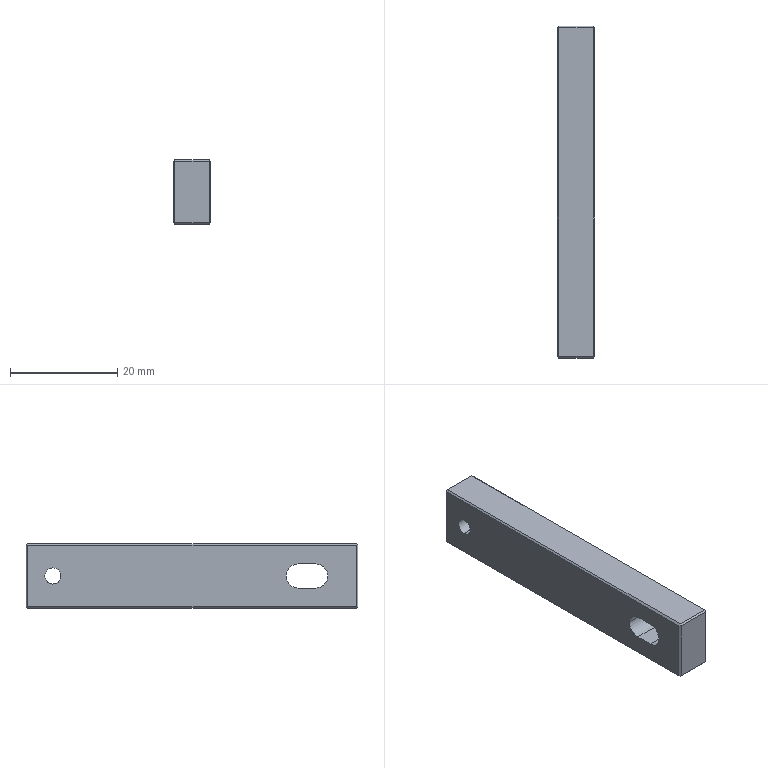Part | NX | 1 solid | 31 faces | box 7 x 62 x 12 mm | volume 4905 mm3 | plane 20 | cylinder 7 | cone 4 | commonest cylinder face diameters 4.5 x3 2.5 x2 3 x2
STEP:
#1=CARTESIAN_POINT('',(-76.,244.,-48.063));
#2=VERTEX_POINT('',#1);
#3=CARTESIAN_POINT('',(-76.,305.4,-48.063));
#4=VERTEX_POINT('',#3);
#5=CARTESIAN_POINT('',(-76.,274.7,-48.063));
#6=DIRECTION('',(0.,1.,0.));
#7=VECTOR('',#6,1000.);
#8=LINE('',#5,#7);
#9=EDGE_CURVE('',#2,#4,#8,.T.);
#10=ORIENTED_EDGE('',*,*,#9,.T.);
#11=CARTESIAN_POINT('',(-76.,305.4,-36.663));
#12=VERTEX_POINT('',#11);
#13=CARTESIAN_POINT('',(-76.,305.4,-42.363));
#14=DIRECTION('',(0.,0.,-1.));
#15=VECTOR('',#14,1000.);
#16=LINE('',#13,#15);
#17=EDGE_CURVE('',#12,#4,#16,.T.);
#18=ORIENTED_EDGE('',*,*,#17,.F.);
#19=CARTESIAN_POINT('',(-76.,244.,-36.663));
#20=VERTEX_POINT('',#19);
#21=CARTESIAN_POINT('',(-76.,274.7,-36.663));
#22=DIRECTION('',(0.,1.,0.));
#23=VECTOR('',#22,1000.);
#24=LINE('',#21,#23);
#25=EDGE_CURVE('',#20,#12,#24,.T.);
#26=ORIENTED_EDGE('',*,*,#25,.F.);
#27=CARTESIAN_POINT('',(-76.,244.,-42.363));
#28=DIRECTION('',(0.,0.,-1.));
#29=VECTOR('',#28,1000.);
#30=LINE('',#27,#29);
#31=EDGE_CURVE('',#20,#2,#30,.T.);
#32=ORIENTED_EDGE('',*,*,#31,.T.);
#33=EDGE_LOOP('',(#10,#18,#26,#32));
#34=FACE_BOUND('',#33,.T.);
#35=CARTESIAN_POINT('',(-76.,251.55,-44.613));
#36=VERTEX_POINT('',#35);
#37=CARTESIAN_POINT('',(-76.,254.85,-44.613));
#38=VERTEX_POINT('',#37);
#39=CARTESIAN_POINT('',(-76.,245.7,-44.613));
#40=DIRECTION('',(0.,1.,0.));
#41=VECTOR('',#40,1000.);
#42=LINE('',#39,#41);
#43=EDGE_CURVE('',#36,#38,#42,.T.);
#44=ORIENTED_EDGE('',*,*,#43,.F.);
#45=CARTESIAN_POINT('',(-76.,251.55,-40.113));
#46=VERTEX_POINT('',#45);
#47=CARTESIAN_POINT('',(-76.,251.55,-42.363));
#48=DIRECTION('',(1.,0.,0.));
#49=DIRECTION('',(0.,1.,0.));
#50=AXIS2_PLACEMENT_3D('',#47,#48,#49);
#51=CIRCLE('',#50,2.25);
#52=EDGE_CURVE('',#46,#36,#51,.T.);
#53=ORIENTED_EDGE('',*,*,#52,.F.);
#54=CARTESIAN_POINT('',(-76.,254.85,-40.113));
#55=VERTEX_POINT('',#54);
#56=CARTESIAN_POINT('',(-76.,245.7,-40.113));
#57=DIRECTION('',(0.,-1.,0.));
#58=VECTOR('',#57,1000.);
#59=LINE('',#56,#58);
#60=EDGE_CURVE('',#55,#46,#59,.T.);
#61=ORIENTED_EDGE('',*,*,#60,.F.);
#62=CARTESIAN_POINT('',(-76.,257.1,-42.363));
#63=VERTEX_POINT('',#62);
#64=CARTESIAN_POINT('',(-76.,254.85,-42.363));
#65=DIRECTION('',(1.,0.,0.));
#66=DIRECTION('',(0.,1.,0.));
#67=AXIS2_PLACEMENT_3D('',#64,#65,#66);
#68=CIRCLE('',#67,2.25);
#69=EDGE_CURVE('',#63,#55,#68,.T.);
#70=ORIENTED_EDGE('',*,*,#69,.F.);
#71=CARTESIAN_POINT('',(-76.,254.85,-42.363));
#72=DIRECTION('',(1.,0.,0.));
#73=DIRECTION('',(0.,1.,0.));
#74=AXIS2_PLACEMENT_3D('',#71,#72,#73);
#75=CIRCLE('',#74,2.25);
#76=EDGE_CURVE('',#38,#63,#75,.T.);
#77=ORIENTED_EDGE('',*,*,#76,.F.);
#78=EDGE_LOOP('',(#44,#53,#61,#70,#77));
#79=FACE_BOUND('',#78,.T.);
#80=CARTESIAN_POINT('',(-76.,302.4,-42.363));
#81=VERTEX_POINT('',#80);
#82=CARTESIAN_POINT('',(-76.,299.,-42.363));
#83=VERTEX_POINT('',#82);
#84=CARTESIAN_POINT('',(-76.,300.7,-42.363));
#85=DIRECTION('',(1.,0.,0.));
#86=DIRECTION('',(0.,0.,-1.));
#87=AXIS2_PLACEMENT_3D('',#84,#85,#86);
#88=CIRCLE('',#87,1.7);
#89=EDGE_CURVE('',#81,#83,#88,.T.);
#90=ORIENTED_EDGE('',*,*,#89,.F.);
#91=CARTESIAN_POINT('',(-76.,300.7,-42.363));
#92=DIRECTION('',(1.,0.,0.));
#93=DIRECTION('',(0.,0.,-1.));
#94=AXIS2_PLACEMENT_3D('',#91,#92,#93);
#95=CIRCLE('',#94,1.7);
#96=EDGE_CURVE('',#83,#81,#95,.T.);
#97=ORIENTED_EDGE('',*,*,#96,.F.);
#98=EDGE_LOOP('',(#90,#97));
#99=FACE_BOUND('',#98,.T.);
#100=CARTESIAN_POINT('',(-76.,245.7,-48.363));
#101=DIRECTION('',(1.,0.,0.));
#102=DIRECTION('',(0.,1.,0.));
#103=AXIS2_PLACEMENT_3D('',#100,#101,#102);
#104=PLANE('',#103);
#105=ADVANCED_FACE('',(#34,#79,#99),#104,.T.);
#106=CARTESIAN_POINT('',(-82.7,305.4,-48.363));
#107=VERTEX_POINT('',#106);
#108=CARTESIAN_POINT('',(-82.7,244.,-48.363));
#109=VERTEX_POINT('',#108);
#110=CARTESIAN_POINT('',(-82.7,0.,-48.363));
#111=DIRECTION('',(0.,-1.,0.));
#112=VECTOR('',#111,1000.);
#113=LINE('',#110,#112);
#114=EDGE_CURVE('',#107,#109,#113,.T.);
#115=ORIENTED_EDGE('',*,*,#114,.F.);
#116=CARTESIAN_POINT('',(-76.3,305.4,-48.363));
#117=VERTEX_POINT('',#116);
#118=CARTESIAN_POINT('',(0.,305.4,-48.363));
#119=DIRECTION('',(-1.,0.,0.));
#120=VECTOR('',#119,1000.);
#121=LINE('',#118,#120);
#122=EDGE_CURVE('',#117,#107,#121,.T.);
#123=ORIENTED_EDGE('',*,*,#122,.F.);
#124=CARTESIAN_POINT('',(-76.3,244.,-48.363));
#125=VERTEX_POINT('',#124);
#126=CARTESIAN_POINT('',(-76.3,0.,-48.363));
#127=DIRECTION('',(0.,1.,0.));
#128=VECTOR('',#127,1000.);
#129=LINE('',#126,#128);
#130=EDGE_CURVE('',#125,#117,#129,.T.);
#131=ORIENTED_EDGE('',*,*,#130,.F.);
#132=CARTESIAN_POINT('',(0.,244.,-48.363));
#133=DIRECTION('',(-1.,0.,0.));
#134=VECTOR('',#133,1000.);
#135=LINE('',#132,#134);
#136=EDGE_CURVE('',#125,#109,#135,.T.);
#137=ORIENTED_EDGE('',*,*,#136,.T.);
#138=EDGE_LOOP('',(#115,#123,#131,#137));
#139=FACE_BOUND('',#138,.T.);
#140=CARTESIAN_POINT('',(-77.8,300.7,-48.363));
#141=VERTEX_POINT('',#140);
#142=CARTESIAN_POINT('',(-81.2,300.7,-48.363));
#143=VERTEX_POINT('',#142);
#144=CARTESIAN_POINT('',(-79.5,300.7,-48.363));
#145=DIRECTION('',(0.,0.,-1.));
#146=DIRECTION('',(-1.,0.,0.));
#147=AXIS2_PLACEMENT_3D('',#144,#145,#146);
#148=CIRCLE('',#147,1.7);
#149=EDGE_CURVE('',#141,#143,#148,.T.);
#150=ORIENTED_EDGE('',*,*,#149,.F.);
#151=CARTESIAN_POINT('',(-79.5,300.7,-48.363));
#152=DIRECTION('',(0.,0.,-1.));
#153=DIRECTION('',(-1.,0.,0.));
#154=AXIS2_PLACEMENT_3D('',#151,#152,#153);
#155=CIRCLE('',#154,1.7);
#156=EDGE_CURVE('',#143,#141,#155,.T.);
#157=ORIENTED_EDGE('',*,*,#156,.F.);
#158=EDGE_LOOP('',(#150,#157));
#159=FACE_BOUND('',#158,.T.);
#160=CARTESIAN_POINT('',(-83.,245.7,-48.363));
#161=DIRECTION('',(0.,0.,-1.));
#162=DIRECTION('',(0.,-1.,0.));
#163=AXIS2_PLACEMENT_3D('',#160,#161,#162);
#164=PLANE('',#163);
#165=ADVANCED_FACE('',(#139,#159),#164,.T.);
#166=CARTESIAN_POINT('',(-83.,244.,-36.663));
#167=VERTEX_POINT('',#166);
#168=CARTESIAN_POINT('',(-83.,305.4,-36.663));
#169=VERTEX_POINT('',#168);
#170=CARTESIAN_POINT('',(-83.,274.7,-36.663));
#171=DIRECTION('',(0.,1.,0.));
#172=VECTOR('',#171,1000.);
#173=LINE('',#170,#172);
#174=EDGE_CURVE('',#167,#169,#173,.T.);
#175=ORIENTED_EDGE('',*,*,#174,.T.);
#176=CARTESIAN_POINT('',(-83.,305.4,-48.063));
#177=VERTEX_POINT('',#176);
#178=CARTESIAN_POINT('',(-83.,305.4,-42.363));
#179=DIRECTION('',(0.,0.,1.));
#180=VECTOR('',#179,1000.);
#181=LINE('',#178,#180);
#182=EDGE_CURVE('',#177,#169,#181,.T.);
#183=ORIENTED_EDGE('',*,*,#182,.F.);
#184=CARTESIAN_POINT('',(-83.,244.,-48.063));
#185=VERTEX_POINT('',#184);
#186=CARTESIAN_POINT('',(-83.,274.7,-48.063));
#187=DIRECTION('',(0.,1.,0.));
#188=VECTOR('',#187,1000.);
#189=LINE('',#186,#188);
#190=EDGE_CURVE('',#185,#177,#189,.T.);
#191=ORIENTED_EDGE('',*,*,#190,.F.);
#192=CARTESIAN_POINT('',(-83.,244.,-42.363));
#193=DIRECTION('',(0.,0.,1.));
#194=VECTOR('',#193,1000.);
#195=LINE('',#192,#194);
#196=EDGE_CURVE('',#185,#167,#195,.T.);
#197=ORIENTED_EDGE('',*,*,#196,.T.);
#198=EDGE_LOOP('',(#175,#183,#191,#197));
#199=FACE_BOUND('',#198,.T.);
#200=CARTESIAN_POINT('',(-83.,300.7,-40.863));
#201=VERTEX_POINT('',#200);
#202=CARTESIAN_POINT('',(-83.,300.7,-43.863));
#203=VERTEX_POINT('',#202);
#204=CARTESIAN_POINT('',(-83.,300.7,-42.363));
#205=DIRECTION('',(1.,0.,0.));
#206=DIRECTION('',(0.,0.,-1.));
#207=AXIS2_PLACEMENT_3D('',#204,#205,#206);
#208=CIRCLE('',#207,1.5);
#209=EDGE_CURVE('',#201,#203,#208,.T.);
#210=ORIENTED_EDGE('',*,*,#209,.T.);
#211=CARTESIAN_POINT('',(-83.,300.7,-42.363));
#212=DIRECTION('',(1.,0.,0.));
#213=DIRECTION('',(0.,0.,-1.));
#214=AXIS2_PLACEMENT_3D('',#211,#212,#213);
#215=CIRCLE('',#214,1.5);
#216=EDGE_CURVE('',#203,#201,#215,.T.);
#217=ORIENTED_EDGE('',*,*,#216,.T.);
#218=EDGE_LOOP('',(#210,#217));
#219=FACE_BOUND('',#218,.T.);
#220=CARTESIAN_POINT('',(-83.,251.55,-40.113));
#221=VERTEX_POINT('',#220);
#222=CARTESIAN_POINT('',(-83.,254.85,-40.113));
#223=VERTEX_POINT('',#222);
#224=CARTESIAN_POINT('',(-83.,245.7,-40.113));
#225=DIRECTION('',(0.,1.,0.));
#226=VECTOR('',#225,1000.);
#227=LINE('',#224,#226);
#228=EDGE_CURVE('',#221,#223,#227,.T.);
#229=ORIENTED_EDGE('',*,*,#228,.F.);
#230=CARTESIAN_POINT('',(-83.,251.55,-44.613));
#231=VERTEX_POINT('',#230);
#232=CARTESIAN_POINT('',(-83.,251.55,-42.363));
#233=DIRECTION('',(1.,0.,0.));
#234=DIRECTION('',(0.,1.,0.));
#235=AXIS2_PLACEMENT_3D('',#232,#233,#234);
#236=CIRCLE('',#235,2.25);
#237=EDGE_CURVE('',#221,#231,#236,.T.);
#238=ORIENTED_EDGE('',*,*,#237,.T.);
#239=CARTESIAN_POINT('',(-83.,254.85,-44.613));
#240=VERTEX_POINT('',#239);
#241=CARTESIAN_POINT('',(-83.,245.7,-44.613));
#242=DIRECTION('',(0.,-1.,0.));
#243=VECTOR('',#242,1000.);
#244=LINE('',#241,#243);
#245=EDGE_CURVE('',#240,#231,#244,.T.);
#246=ORIENTED_EDGE('',*,*,#245,.F.);
#247=CARTESIAN_POINT('',(-83.,257.1,-42.363));
#248=VERTEX_POINT('',#247);
#249=CARTESIAN_POINT('',(-83.,254.85,-42.363));
#250=DIRECTION('',(1.,0.,0.));
#251=DIRECTION('',(0.,1.,0.));
#252=AXIS2_PLACEMENT_3D('',#249,#250,#251);
#253=CIRCLE('',#252,2.25);
#254=EDGE_CURVE('',#240,#248,#253,.T.);
#255=ORIENTED_EDGE('',*,*,#254,.T.);
#256=CARTESIAN_POINT('',(-83.,254.85,-42.363));
#257=DIRECTION('',(1.,0.,0.));
#258=DIRECTION('',(0.,1.,0.));
#259=AXIS2_PLACEMENT_3D('',#256,#257,#258);
#260=CIRCLE('',#259,2.25);
#261=EDGE_CURVE('',#248,#223,#260,.T.);
#262=ORIENTED_EDGE('',*,*,#261,.T.);
#263=EDGE_LOOP('',(#229,#238,#246,#255,#262));
#264=FACE_BOUND('',#263,.T.);
#265=CARTESIAN_POINT('',(-83.,245.7,-36.363));
#266=DIRECTION('',(-1.,0.,0.));
#267=DIRECTION('',(0.,0.,1.));
#268=AXIS2_PLACEMENT_3D('',#265,#266,#267);
#269=PLANE('',#268);
#270=ADVANCED_FACE('',(#199,#219,#264),#269,.T.);
#271=CARTESIAN_POINT('',(-82.7,244.,-36.363));
#272=VERTEX_POINT('',#271);
#273=CARTESIAN_POINT('',(-76.3,244.,-36.363));
#274=VERTEX_POINT('',#273);
#275=CARTESIAN_POINT('',(-79.5,244.,-36.363));
#276=DIRECTION('',(1.,0.,0.));
#277=VECTOR('',#276,1000.);
#278=LINE('',#275,#277);
#279=EDGE_CURVE('',#272,#274,#278,.T.);
#280=ORIENTED_EDGE('',*,*,#279,.T.);
#281=CARTESIAN_POINT('',(-76.3,305.4,-36.363));
#282=VERTEX_POINT('',#281);
#283=CARTESIAN_POINT('',(-76.3,274.7,-36.363));
#284=DIRECTION('',(0.,1.,0.));
#285=VECTOR('',#284,1000.);
#286=LINE('',#283,#285);
#287=EDGE_CURVE('',#274,#282,#286,.T.);
#288=ORIENTED_EDGE('',*,*,#287,.T.);
#289=CARTESIAN_POINT('',(-82.7,305.4,-36.363));
#290=VERTEX_POINT('',#289);
#291=CARTESIAN_POINT('',(-79.5,305.4,-36.363));
#292=DIRECTION('',(1.,0.,0.));
#293=VECTOR('',#292,1000.);
#294=LINE('',#291,#293);
#295=EDGE_CURVE('',#290,#282,#294,.T.);
#296=ORIENTED_EDGE('',*,*,#295,.F.);
#297=CARTESIAN_POINT('',(-82.7,274.7,-36.363));
#298=DIRECTION('',(0.,1.,0.));
#299=VECTOR('',#298,1000.);
#300=LINE('',#297,#299);
#301=EDGE_CURVE('',#272,#290,#300,.T.);
#302=ORIENTED_EDGE('',*,*,#301,.F.);
#303=EDGE_LOOP('',(#280,#288,#296,#302));
#304=FACE_BOUND('',#303,.T.);
#305=CARTESIAN_POINT('',(-76.,245.7,-36.363));
#306=DIRECTION('',(0.,0.,1.));
#307=DIRECTION('',(1.,0.,0.));
#308=AXIS2_PLACEMENT_3D('',#305,#306,#307);
#309=PLANE('',#308);
#310=ADVANCED_FACE('',(#304),#309,.T.);
#311=CARTESIAN_POINT('',(-83.7,257.1,-42.363));
#312=DIRECTION('',(1.,0.,0.));
#313=VECTOR('',#312,1000.);
#314=LINE('',#311,#313);
#315=EDGE_CURVE('',#248,#63,#314,.T.);
#316=ORIENTED_EDGE('',*,*,#315,.F.);
#317=ORIENTED_EDGE('',*,*,#254,.F.);
#318=CARTESIAN_POINT('',(-83.7,254.85,-44.613));
#319=DIRECTION('',(1.,0.,0.));
#320=VECTOR('',#319,1000.);
#321=LINE('',#318,#320);
#322=EDGE_CURVE('',#240,#38,#321,.T.);
#323=ORIENTED_EDGE('',*,*,#322,.T.);
#324=ORIENTED_EDGE('',*,*,#76,.T.);
#325=EDGE_LOOP('',(#316,#317,#323,#324));
#326=FACE_BOUND('',#325,.T.);
#327=CARTESIAN_POINT('',(-83.7,254.85,-42.363));
#328=DIRECTION('',(1.,0.,0.));
#329=DIRECTION('',(0.,1.,0.));
#330=AXIS2_PLACEMENT_3D('',#327,#328,#329);
#331=CYLINDRICAL_SURFACE('',#330,2.25);
#332=ADVANCED_FACE('',(#326),#331,.F.);
#333=ORIENTED_EDGE('',*,*,#237,.F.);
#334=CARTESIAN_POINT('',(-83.7,251.55,-40.113));
#335=DIRECTION('',(1.,0.,0.));
#336=VECTOR('',#335,1000.);
#337=LINE('',#334,#336);
#338=EDGE_CURVE('',#221,#46,#337,.T.);
#339=ORIENTED_EDGE('',*,*,#338,.T.);
#340=ORIENTED_EDGE('',*,*,#52,.T.);
#341=CARTESIAN_POINT('',(-83.7,251.55,-44.613));
#342=DIRECTION('',(1.,0.,0.));
#343=VECTOR('',#342,1000.);
#344=LINE('',#341,#343);
#345=EDGE_CURVE('',#231,#36,#344,.T.);
#346=ORIENTED_EDGE('',*,*,#345,.F.);
#347=EDGE_LOOP('',(#333,#339,#340,#346));
#348=FACE_BOUND('',#347,.T.);
#349=CARTESIAN_POINT('',(-83.7,251.55,-42.363));
#350=DIRECTION('',(1.,0.,0.));
#351=DIRECTION('',(0.,1.,0.));
#352=AXIS2_PLACEMENT_3D('',#349,#350,#351);
#353=CYLINDRICAL_SURFACE('',#352,2.25);
#354=ADVANCED_FACE('',(#348),#353,.F.);
#355=ORIENTED_EDGE('',*,*,#245,.T.);
#356=ORIENTED_EDGE('',*,*,#345,.T.);
#357=ORIENTED_EDGE('',*,*,#43,.T.);
#358=ORIENTED_EDGE('',*,*,#322,.F.);
#359=EDGE_LOOP('',(#355,#356,#357,#358));
#360=FACE_BOUND('',#359,.T.);
#361=CARTESIAN_POINT('',(-83.7,254.85,-44.613));
#362=DIRECTION('',(0.,0.,-1.));
#363=DIRECTION('',(-1.,0.,0.));
#364=AXIS2_PLACEMENT_3D('',#361,#362,#363);
#365=PLANE('',#364);
#366=ADVANCED_FACE('',(#360),#365,.F.);
#367=ORIENTED_EDGE('',*,*,#228,.T.);
#368=CARTESIAN_POINT('',(-83.7,254.85,-40.113));
#369=DIRECTION('',(1.,0.,0.));
#370=VECTOR('',#369,1000.);
#371=LINE('',#368,#370);
#372=EDGE_CURVE('',#223,#55,#371,.T.);
#373=ORIENTED_EDGE('',*,*,#372,.T.);
#374=ORIENTED_EDGE('',*,*,#60,.T.);
#375=ORIENTED_EDGE('',*,*,#338,.F.);
#376=EDGE_LOOP('',(#367,#373,#374,#375));
#377=FACE_BOUND('',#376,.T.);
#378=CARTESIAN_POINT('',(-83.7,251.55,-40.113));
#379=DIRECTION('',(0.,0.,1.));
#380=DIRECTION('',(1.,0.,0.));
#381=AXIS2_PLACEMENT_3D('',#378,#379,#380);
#382=PLANE('',#381);
#383=ADVANCED_FACE('',(#377),#382,.F.);
#384=CARTESIAN_POINT('',(-76.2,299.2,-42.363));
#385=VERTEX_POINT('',#384);
#386=CARTESIAN_POINT('',(-76.2,300.7,-43.863));
#387=VERTEX_POINT('',#386);
#388=CARTESIAN_POINT('',(-76.2,300.7,-42.363));
#389=DIRECTION('',(1.,0.,0.));
#390=DIRECTION('',(0.,-1.,0.));
#391=AXIS2_PLACEMENT_3D('',#388,#389,#390);
#392=CIRCLE('',#391,1.5);
#393=EDGE_CURVE('',#385,#387,#392,.T.);
#394=ORIENTED_EDGE('',*,*,#393,.T.);
#395=CARTESIAN_POINT('',(-78.25,300.7,-43.863));
#396=VERTEX_POINT('',#395);
#397=CARTESIAN_POINT('',(-76.,300.7,-43.863));
#398=DIRECTION('',(1.,0.,0.));
#399=VECTOR('',#398,1000.);
#400=LINE('',#397,#399);
#401=EDGE_CURVE('',#396,#387,#400,.T.);
#402=ORIENTED_EDGE('',*,*,#401,.F.);
#403=CARTESIAN_POINT('',(-80.75,300.7,-43.863));
#404=VERTEX_POINT('',#403);
#405=CARTESIAN_POINT('',(-78.25,300.7,-43.863));
#406=CARTESIAN_POINT('',(-78.25,300.672,-43.863));
#407=CARTESIAN_POINT('',(-78.251,300.645,-43.862));
#408=CARTESIAN_POINT('',(-78.253,300.617,-43.861));
#409=CARTESIAN_POINT('',(-78.254,300.602,-43.86));
#410=CARTESIAN_POINT('',(-78.255,300.587,-43.859));
#411=CARTESIAN_POINT('',(-78.257,300.572,-43.858));
#412=CARTESIAN_POINT('',(-78.258,300.557,-43.856));
#413=CARTESIAN_POINT('',(-78.26,300.542,-43.855));
#414=CARTESIAN_POINT('',(-78.262,300.527,-43.853));
#415=CARTESIAN_POINT('',(-78.266,300.497,-43.85));
#416=CARTESIAN_POINT('',(-78.271,300.468,-43.845));
#417=CARTESIAN_POINT('',(-78.278,300.439,-43.84));
#418=CARTESIAN_POINT('',(-78.284,300.409,-43.835));
#419=CARTESIAN_POINT('',(-78.291,300.38,-43.829));
#420=CARTESIAN_POINT('',(-78.299,300.352,-43.822));
#421=CARTESIAN_POINT('',(-78.308,300.323,-43.815));
#422=CARTESIAN_POINT('',(-78.317,300.296,-43.808));
#423=CARTESIAN_POINT('',(-78.327,300.268,-43.8));
#424=CARTESIAN_POINT('',(-78.337,300.241,-43.791));
#425=CARTESIAN_POINT('',(-78.348,300.214,-43.783));
#426=CARTESIAN_POINT('',(-78.36,300.188,-43.773));
#427=CARTESIAN_POINT('',(-78.371,300.162,-43.763));
#428=CARTESIAN_POINT('',(-78.384,300.136,-43.753));
#429=CARTESIAN_POINT('',(-78.397,300.111,-43.743));
#430=CARTESIAN_POINT('',(-78.411,300.086,-43.732));
#431=CARTESIAN_POINT('',(-78.425,300.062,-43.721));
#432=CARTESIAN_POINT('',(-78.44,300.038,-43.709));
#433=CARTESIAN_POINT('',(-78.455,300.014,-43.697));
#434=CARTESIAN_POINT('',(-78.47,299.991,-43.685));
#435=CARTESIAN_POINT('',(-78.486,299.968,-43.673));
#436=CARTESIAN_POINT('',(-78.504,299.943,-43.659));
#437=CARTESIAN_POINT('',(-78.523,299.919,-43.644));
#438=CARTESIAN_POINT('',(-78.543,299.896,-43.629));
#439=CARTESIAN_POINT('',(-78.562,299.873,-43.615));
#440=CARTESIAN_POINT('',(-78.582,299.851,-43.6));
#441=CARTESIAN_POINT('',(-78.603,299.829,-43.584));
#442=CARTESIAN_POINT('',(-78.624,299.808,-43.569));
#443=CARTESIAN_POINT('',(-78.646,299.787,-43.553));
#444=CARTESIAN_POINT('',(-78.668,299.767,-43.537));
#445=CARTESIAN_POINT('',(-78.691,299.747,-43.522));
#446=CARTESIAN_POINT('',(-78.714,299.728,-43.506));
#447=CARTESIAN_POINT('',(-78.737,299.71,-43.49));
#448=CARTESIAN_POINT('',(-78.761,299.691,-43.474));
#449=CARTESIAN_POINT('',(-78.785,299.674,-43.458));
#450=CARTESIAN_POINT('',(-78.81,299.658,-43.442));
#451=CARTESIAN_POINT('',(-78.835,299.641,-43.426));
#452=CARTESIAN_POINT('',(-78.861,299.625,-43.41));
#453=CARTESIAN_POINT('',(-78.887,299.611,-43.394));
#454=CARTESIAN_POINT('',(-78.9,299.603,-43.387));
#455=CARTESIAN_POINT('',(-78.913,299.596,-43.379));
#456=CARTESIAN_POINT('',(-78.926,299.589,-43.371));
#457=CARTESIAN_POINT('',(-78.94,299.582,-43.364));
#458=CARTESIAN_POINT('',(-78.953,299.576,-43.356));
#459=CARTESIAN_POINT('',(-78.967,299.569,-43.349));
#460=CARTESIAN_POINT('',(-78.994,299.556,-43.334));
#461=CARTESIAN_POINT('',(-79.022,299.544,-43.32));
#462=CARTESIAN_POINT('',(-79.051,299.533,-43.306));
#463=CARTESIAN_POINT('',(-79.068,299.527,-43.298));
#464=CARTESIAN_POINT('',(-79.085,299.521,-43.29));
#465=CARTESIAN_POINT('',(-79.103,299.515,-43.282));
#466=CARTESIAN_POINT('',(-79.12,299.509,-43.275));
#467=CARTESIAN_POINT('',(-79.138,299.503,-43.268));
#468=CARTESIAN_POINT('',(-79.156,299.498,-43.261));
#469=CARTESIAN_POINT('',(-79.192,299.488,-43.247));
#470=CARTESIAN_POINT('',(-79.228,299.479,-43.235));
#471=CARTESIAN_POINT('',(-79.266,299.472,-43.225));
#472=CARTESIAN_POINT('',(-79.285,299.469,-43.22));
#473=CARTESIAN_POINT('',(-79.304,299.465,-43.215));
#474=CARTESIAN_POINT('',(-79.323,299.463,-43.211));
#475=CARTESIAN_POINT('',(-79.342,299.46,-43.207));
#476=CARTESIAN_POINT('',(-79.362,299.458,-43.203));
#477=CARTESIAN_POINT('',(-79.381,299.456,-43.201));
#478=CARTESIAN_POINT('',(-79.401,299.454,-43.198));
#479=CARTESIAN_POINT('',(-79.421,299.452,-43.196));
#480=CARTESIAN_POINT('',(-79.44,299.451,-43.194));
#481=CARTESIAN_POINT('',(-79.46,299.45,-43.193));
#482=CARTESIAN_POINT('',(-79.48,299.45,-43.192));
#483=CARTESIAN_POINT('',(-79.5,299.45,-43.192));
#484=CARTESIAN_POINT('',(-79.519,299.45,-43.192));
#485=CARTESIAN_POINT('',(-79.539,299.45,-43.193));
#486=CARTESIAN_POINT('',(-79.559,299.451,-43.194));
#487=CARTESIAN_POINT('',(-79.579,299.452,-43.196));
#488=CARTESIAN_POINT('',(-79.598,299.454,-43.198));
#489=CARTESIAN_POINT('',(-79.618,299.456,-43.201));
#490=CARTESIAN_POINT('',(-79.638,299.457,-43.203));
#491=CARTESIAN_POINT('',(-79.657,299.46,-43.207));
#492=CARTESIAN_POINT('',(-79.676,299.463,-43.211));
#493=CARTESIAN_POINT('',(-79.696,299.465,-43.215));
#494=CARTESIAN_POINT('',(-79.715,299.468,-43.219));
#495=CARTESIAN_POINT('',(-79.734,299.472,-43.225));
#496=CARTESIAN_POINT('',(-79.743,299.474,-43.227));
#497=CARTESIAN_POINT('',(-79.752,299.476,-43.23));
#498=CARTESIAN_POINT('',(-79.762,299.478,-43.233));
#499=CARTESIAN_POINT('',(-79.771,299.48,-43.235));
#500=CARTESIAN_POINT('',(-79.78,299.482,-43.238));
#501=CARTESIAN_POINT('',(-79.789,299.484,-43.241));
#502=CARTESIAN_POINT('',(-79.808,299.488,-43.247));
#503=CARTESIAN_POINT('',(-79.826,299.493,-43.254));
#504=CARTESIAN_POINT('',(-79.844,299.498,-43.261));
#505=CARTESIAN_POINT('',(-79.861,299.503,-43.267));
#506=CARTESIAN_POINT('',(-79.879,299.509,-43.275));
#507=CARTESIAN_POINT('',(-79.897,299.515,-43.282));
#508=CARTESIAN_POINT('',(-79.914,299.52,-43.29));
#509=CARTESIAN_POINT('',(-79.931,299.527,-43.297));
#510=CARTESIAN_POINT('',(-79.948,299.533,-43.306));
#511=CARTESIAN_POINT('',(-79.977,299.544,-43.319));
#512=CARTESIAN_POINT('',(-80.005,299.556,-43.334));
#513=CARTESIAN_POINT('',(-80.033,299.569,-43.349));
#514=CARTESIAN_POINT('',(-80.046,299.576,-43.356));
#515=CARTESIAN_POINT('',(-80.06,299.582,-43.363));
#516=CARTESIAN_POINT('',(-80.073,299.589,-43.371));
#517=CARTESIAN_POINT('',(-80.086,299.596,-43.379));
#518=CARTESIAN_POINT('',(-80.1,299.603,-43.386));
#519=CARTESIAN_POINT('',(-80.113,299.61,-43.394));
#520=CARTESIAN_POINT('',(-80.139,299.625,-43.41));
#521=CARTESIAN_POINT('',(-80.164,299.641,-43.425));
#522=CARTESIAN_POINT('',(-80.189,299.657,-43.441));
#523=CARTESIAN_POINT('',(-80.214,299.674,-43.457));
#524=CARTESIAN_POINT('',(-80.238,299.691,-43.473));
#525=CARTESIAN_POINT('',(-80.262,299.709,-43.489));
#526=CARTESIAN_POINT('',(-80.286,299.727,-43.505));
#527=CARTESIAN_POINT('',(-80.309,299.747,-43.521));
#528=CARTESIAN_POINT('',(-80.331,299.766,-43.537));
#529=CARTESIAN_POINT('',(-80.354,299.786,-43.553));
#530=CARTESIAN_POINT('',(-80.375,299.807,-43.569));
#531=CARTESIAN_POINT('',(-80.396,299.829,-43.584));
#532=CARTESIAN_POINT('',(-80.417,299.85,-43.599));
#533=CARTESIAN_POINT('',(-80.438,299.873,-43.615));
#534=CARTESIAN_POINT('',(-80.457,299.896,-43.629));
#535=CARTESIAN_POINT('',(-80.467,299.907,-43.637));
#536=CARTESIAN_POINT('',(-80.476,299.919,-43.644));
#537=CARTESIAN_POINT('',(-80.486,299.931,-43.651));
#538=CARTESIAN_POINT('',(-80.495,299.943,-43.658));
#539=CARTESIAN_POINT('',(-80.504,299.956,-43.665));
#540=CARTESIAN_POINT('',(-80.513,299.968,-43.672));
#541=CARTESIAN_POINT('',(-80.529,299.99,-43.685));
#542=CARTESIAN_POINT('',(-80.545,300.014,-43.697));
#543=CARTESIAN_POINT('',(-80.56,300.037,-43.709));
#544=CARTESIAN_POINT('',(-80.575,300.061,-43.72));
#545=CARTESIAN_POINT('',(-80.589,300.086,-43.732));
#546=CARTESIAN_POINT('',(-80.602,300.111,-43.742));
#547=CARTESIAN_POINT('',(-80.616,300.136,-43.753));
#548=CARTESIAN_POINT('',(-80.628,300.162,-43.763));
#549=CARTESIAN_POINT('',(-80.64,300.188,-43.773));
#550=CARTESIAN_POINT('',(-80.652,300.214,-43.782));
#551=CARTESIAN_POINT('',(-80.663,300.241,-43.791));
#552=CARTESIAN_POINT('',(-80.673,300.268,-43.8));
#553=CARTESIAN_POINT('',(-80.678,300.282,-43.804));
#554=CARTESIAN_POINT('',(-80.683,300.295,-43.808));
#555=CARTESIAN_POINT('',(-80.687,300.309,-43.811));
#556=CARTESIAN_POINT('',(-80.692,300.323,-43.815));
#557=CARTESIAN_POINT('',(-80.696,300.337,-43.819));
#558=CARTESIAN_POINT('',(-80.7,300.351,-43.822));
#559=CARTESIAN_POINT('',(-80.709,300.38,-43.829));
#560=CARTESIAN_POINT('',(-80.716,300.409,-43.835));
#561=CARTESIAN_POINT('',(-80.722,300.438,-43.84));
#562=CARTESIAN_POINT('',(-80.725,300.453,-43.843));
#563=CARTESIAN_POINT('',(-80.728,300.467,-43.845));
#564=CARTESIAN_POINT('',(-80.731,300.482,-43.847));
#565=CARTESIAN_POINT('',(-80.734,300.497,-43.849));
#566=CARTESIAN_POINT('',(-80.736,300.512,-43.851));
#567=CARTESIAN_POINT('',(-80.738,300.527,-43.853));
#568=CARTESIAN_POINT('',(-80.74,300.542,-43.855));
#569=CARTESIAN_POINT('',(-80.742,300.557,-43.856));
#570=CARTESIAN_POINT('',(-80.743,300.572,-43.858));
#571=CARTESIAN_POINT('',(-80.745,300.587,-43.859));
#572=CARTESIAN_POINT('',(-80.746,300.602,-43.86));
#573=CARTESIAN_POINT('',(-80.747,300.617,-43.861));
#574=CARTESIAN_POINT('',(-80.748,300.631,-43.862));
#575=CARTESIAN_POINT('',(-80.749,300.645,-43.862));
#576=CARTESIAN_POINT('',(-80.749,300.658,-43.862));
#577=CARTESIAN_POINT('',(-80.75,300.672,-43.863));
#578=CARTESIAN_POINT('',(-80.75,300.686,-43.863));
#579=CARTESIAN_POINT('',(-80.75,300.7,-43.863));
#580=B_SPLINE_CURVE_WITH_KNOTS('',3,(#405,#406,#407,#408,#409,#410,#411,#412,#413,#414,#415,#416,#417,#418,#419,#420,#421,#422,#423,#424,#425,#426,#427,#428,#429,#430,#431,#432,#433,#434,#435,#436,#437,#438,#439,#440,#441,#442,#443,#444,#445,#446,#447,#448,#449,#450,#451,#452,#453,#454,#455,#456,#457,#458,#459,#460,#461,#462,#463,#464,#465,#466,#467,#468,#469,#470,#471,#472,#473,#474,#475,#476,#477,#478,#479,#480,#481,#482,#483,#484,#485,#486,#487,#488,#489,#490,#491,#492,#493,#494,#495,#496,#497,#498,#499,#500,#501,#502,#503,#504,#505,#506,#507,#508,#509,#510,#511,#512,#513,#514,#515,#516,#517,#518,#519,#520,#521,#522,#523,#524,#525,#526,#527,#528,#529,#530,#531,#532,#533,#534,#535,#536,#537,#538,#539,#540,#541,#542,#543,#544,#545,#546,#547,#548,#549,#550,#551,#552,#553,#554,#555,#556,#557,#558,#559,#560,#561,#562,#563,#564,#565,#566,#567,#568,#569,#570,#571,#572,#573,#574,#575,#576,#577,#578,#579),.UNSPECIFIED.,.F.,.F.,(4,3,3,3,3,3,3,3,3,3,3,3,3,3,3,3,3,3,3,3,3,3,3,3,3,3,3,3,3,3,3,3,3,3,3,3,3,3,3,3,3,3,3,3,3,3,3,3,3,3,3,3,3,3,3,3,3,3,4),(0.,0.08315,0.1285,0.1738,0.2648,0.3559,0.4468,0.5374,0.6284,0.7196,0.8107,0.912,1.013,1.115,1.216,1.318,1.419,1.47,1.52,1.622,1.681,1.741,1.86,1.919,1.979,2.038,2.098,2.157,2.217,2.276,2.336,2.366,2.395,2.455,2.514,2.574,2.675,2.726,2.776,2.878,2.979,3.081,3.182,3.284,3.334,3.385,3.476,3.567,3.658,3.749,3.794,3.84,3.931,3.976,4.022,4.067,4.113,4.154,4.196),.UNSPECIFIED.);
#581=EDGE_CURVE('',#396,#404,#580,.T.);
#582=ORIENTED_EDGE('',*,*,#581,.T.);
#583=CARTESIAN_POINT('',(-76.,300.7,-43.863));
#584=DIRECTION('',(1.,0.,0.));
#585=VECTOR('',#584,1000.);
#586=LINE('',#583,#585);
#587=EDGE_CURVE('',#203,#404,#586,.T.);
#588=ORIENTED_EDGE('',*,*,#587,.F.);
#589=ORIENTED_EDGE('',*,*,#209,.F.);
#590=CARTESIAN_POINT('',(-76.2,300.7,-40.863));
#591=VERTEX_POINT('',#590);
#592=CARTESIAN_POINT('',(-76.,300.7,-40.863));
#593=DIRECTION('',(1.,0.,0.));
#594=VECTOR('',#593,1000.);
#595=LINE('',#592,#594);
#596=EDGE_CURVE('',#201,#591,#595,.T.);
#597=ORIENTED_EDGE('',*,*,#596,.T.);
#598=CARTESIAN_POINT('',(-76.2,300.7,-42.363));
#599=DIRECTION('',(1.,0.,0.));
#600=DIRECTION('',(0.,-1.,0.));
#601=AXIS2_PLACEMENT_3D('',#598,#599,#600);
#602=CIRCLE('',#601,1.5);
#603=EDGE_CURVE('',#591,#385,#602,.T.);
#604=ORIENTED_EDGE('',*,*,#603,.T.);
#605=EDGE_LOOP('',(#394,#402,#582,#588,#589,#597,#604));
#606=FACE_BOUND('',#605,.T.);
#607=CARTESIAN_POINT('',(-76.,300.7,-42.363));
#608=DIRECTION('',(1.,0.,0.));
#609=DIRECTION('',(0.,0.,-1.));
#610=AXIS2_PLACEMENT_3D('',#607,#608,#609);
#611=CYLINDRICAL_SURFACE('',#610,1.5);
#612=ADVANCED_FACE('',(#606),#611,.F.);
#613=ORIENTED_EDGE('',*,*,#393,.F.);
#614=CARTESIAN_POINT('',(-76.2,299.2,-42.363));
#615=DIRECTION('',(0.7071,-0.7071,0.));
#616=VECTOR('',#615,1000.);
#617=LINE('',#614,#616);
#618=EDGE_CURVE('',#83,#385,#617,.F.);
#619=ORIENTED_EDGE('',*,*,#618,.F.);
#620=ORIENTED_EDGE('',*,*,#96,.T.);
#621=CARTESIAN_POINT('',(-76.2,302.2,-42.363));
#622=VERTEX_POINT('',#621);
#623=CARTESIAN_POINT('',(-76.2,302.2,-42.363));
#624=DIRECTION('',(0.7071,0.7071,0.));
#625=VECTOR('',#624,1000.);
#626=LINE('',#623,#625);
#627=EDGE_CURVE('',#81,#622,#626,.F.);
#628=ORIENTED_EDGE('',*,*,#627,.T.);
#629=CARTESIAN_POINT('',(-76.2,300.7,-42.363));
#630=DIRECTION('',(1.,0.,0.));
#631=DIRECTION('',(0.,-1.,0.));
#632=AXIS2_PLACEMENT_3D('',#629,#630,#631);
#633=CIRCLE('',#632,1.5);
#634=EDGE_CURVE('',#387,#622,#633,.T.);
#635=ORIENTED_EDGE('',*,*,#634,.F.);
#636=EDGE_LOOP('',(#613,#619,#620,#628,#635));
#637=FACE_BOUND('',#636,.T.);
#638=CARTESIAN_POINT('',(-76.2,300.7,-42.363));
#639=DIRECTION('',(1.,0.,0.));
#640=DIRECTION('',(0.,-1.,0.));
#641=AXIS2_PLACEMENT_3D('',#638,#639,#640);
#642=CONICAL_SURFACE('',#641,1.5,0.7854);
#643=ADVANCED_FACE('',(#637),#642,.F.);
#644=CARTESIAN_POINT('',(-82.7,305.7,-36.663));
#645=VERTEX_POINT('',#644);
#646=CARTESIAN_POINT('',(-76.3,305.7,-36.663));
#647=VERTEX_POINT('',#646);
#648=CARTESIAN_POINT('',(-79.5,305.7,-36.663));
#649=DIRECTION('',(1.,0.,0.));
#650=VECTOR('',#649,1000.);
#651=LINE('',#648,#650);
#652=EDGE_CURVE('',#645,#647,#651,.T.);
#653=ORIENTED_EDGE('',*,*,#652,.F.);
#654=CARTESIAN_POINT('',(-82.85,305.55,-36.513));
#655=VERTEX_POINT('',#654);
#656=CARTESIAN_POINT('',(-72.373,316.027,-46.991));
#657=DIRECTION('',(0.5774,0.5774,-0.5774));
#658=VECTOR('',#657,1000.);
#659=LINE('',#656,#658);
#660=EDGE_CURVE('',#655,#645,#659,.T.);
#661=ORIENTED_EDGE('',*,*,#660,.F.);
#662=CARTESIAN_POINT('',(-93.327,316.027,-46.991));
#663=DIRECTION('',(-0.5774,0.5774,-0.5774));
#664=VECTOR('',#663,1000.);
#665=LINE('',#662,#664);
#666=EDGE_CURVE('',#290,#655,#665,.T.);
#667=ORIENTED_EDGE('',*,*,#666,.F.);
#668=ORIENTED_EDGE('',*,*,#295,.T.);
#669=CARTESIAN_POINT('',(-76.15,305.55,-36.513));
#670=VERTEX_POINT('',#669);
#671=CARTESIAN_POINT('',(-65.673,316.027,-46.991));
#672=DIRECTION('',(0.5774,0.5774,-0.5774));
#673=VECTOR('',#672,1000.);
#674=LINE('',#671,#673);
#675=EDGE_CURVE('',#282,#670,#674,.T.);
#676=ORIENTED_EDGE('',*,*,#675,.T.);
#677=CARTESIAN_POINT('',(-86.627,316.027,-46.991));
#678=DIRECTION('',(-0.5774,0.5774,-0.5774));
#679=VECTOR('',#678,1000.);
#680=LINE('',#677,#679);
#681=EDGE_CURVE('',#670,#647,#680,.T.);
#682=ORIENTED_EDGE('',*,*,#681,.T.);
#683=EDGE_LOOP('',(#653,#661,#667,#668,#676,#682));
#684=FACE_BOUND('',#683,.T.);
#685=CARTESIAN_POINT('',(-79.5,305.55,-36.513));
#686=DIRECTION('',(0.,0.7071,0.7071));
#687=DIRECTION('',(1.,0.,0.));
#688=AXIS2_PLACEMENT_3D('',#685,#686,#687);
#689=PLANE('',#688);
#690=ADVANCED_FACE('',(#684),#689,.T.);
#691=CARTESIAN_POINT('',(-82.7,305.7,-48.063));
#692=VERTEX_POINT('',#691);
#693=CARTESIAN_POINT('',(-82.7,305.7,-42.363));
#694=DIRECTION('',(0.,0.,1.));
#695=VECTOR('',#694,1000.);
#696=LINE('',#693,#695);
#697=EDGE_CURVE('',#692,#645,#696,.T.);
#698=ORIENTED_EDGE('',*,*,#697,.F.);
#699=CARTESIAN_POINT('',(-82.85,305.55,-48.213));
#700=VERTEX_POINT('',#699);
#701=CARTESIAN_POINT('',(-81.627,306.773,-46.991));
#702=DIRECTION('',(0.5774,0.5774,0.5774));
#703=VECTOR('',#702,1000.);
#704=LINE('',#701,#703);
#705=EDGE_CURVE('',#700,#692,#704,.T.);
#706=ORIENTED_EDGE('',*,*,#705,.F.);
#707=CARTESIAN_POINT('',(-84.073,304.327,-46.991));
#708=DIRECTION('',(0.5774,0.5774,-0.5774));
#709=VECTOR('',#708,1000.);
#710=LINE('',#707,#709);
#711=EDGE_CURVE('',#177,#700,#710,.T.);
#712=ORIENTED_EDGE('',*,*,#711,.F.);
#713=ORIENTED_EDGE('',*,*,#182,.T.);
#714=CARTESIAN_POINT('',(-93.327,295.073,-46.991));
#715=DIRECTION('',(0.5774,0.5774,0.5774));
#716=VECTOR('',#715,1000.);
#717=LINE('',#714,#716);
#718=EDGE_CURVE('',#169,#655,#717,.T.);
#719=ORIENTED_EDGE('',*,*,#718,.T.);
#720=ORIENTED_EDGE('',*,*,#660,.T.);
#721=EDGE_LOOP('',(#698,#706,#712,#713,#719,#720));
#722=FACE_BOUND('',#721,.T.);
#723=CARTESIAN_POINT('',(-82.85,305.55,-42.363));
#724=DIRECTION('',(-0.7071,0.7071,0.));
#725=DIRECTION('',(0.,0.,1.));
#726=AXIS2_PLACEMENT_3D('',#723,#724,#725);
#727=PLANE('',#726);
#728=ADVANCED_FACE('',(#722),#727,.T.);
#729=ORIENTED_EDGE('',*,*,#25,.T.);
#730=CARTESIAN_POINT('',(-86.393,315.793,-26.27));
#731=DIRECTION('',(0.5774,-0.5774,-0.5774));
#732=VECTOR('',#731,1000.);
#733=LINE('',#730,#732);
#734=EDGE_CURVE('',#670,#12,#733,.T.);
#735=ORIENTED_EDGE('',*,*,#734,.F.);
#736=ORIENTED_EDGE('',*,*,#675,.F.);
#737=ORIENTED_EDGE('',*,*,#287,.F.);
#738=CARTESIAN_POINT('',(-76.15,243.85,-36.513));
#739=VERTEX_POINT('',#738);
#740=CARTESIAN_POINT('',(-65.673,233.373,-46.991));
#741=DIRECTION('',(0.5774,-0.5774,-0.5774));
#742=VECTOR('',#741,1000.);
#743=LINE('',#740,#742);
#744=EDGE_CURVE('',#274,#739,#743,.T.);
#745=ORIENTED_EDGE('',*,*,#744,.T.);
#746=CARTESIAN_POINT('',(-86.393,233.607,-26.27));
#747=DIRECTION('',(0.5774,0.5774,-0.5774));
#748=VECTOR('',#747,1000.);
#749=LINE('',#746,#748);
#750=EDGE_CURVE('',#739,#20,#749,.T.);
#751=ORIENTED_EDGE('',*,*,#750,.T.);
#752=EDGE_LOOP('',(#729,#735,#736,#737,#745,#751));
#753=FACE_BOUND('',#752,.T.);
#754=CARTESIAN_POINT('',(-76.15,274.7,-36.513));
#755=DIRECTION('',(-0.7071,0.,-0.7071));
#756=DIRECTION('',(-0.7071,0.,0.7071));
#757=AXIS2_PLACEMENT_3D('',#754,#755,#756);
#758=PLANE('',#757);
#759=ADVANCED_FACE('',(#753),#758,.F.);
#760=ORIENTED_EDGE('',*,*,#9,.F.);
#761=CARTESIAN_POINT('',(-76.15,243.85,-48.213));
#762=VERTEX_POINT('',#761);
#763=CARTESIAN_POINT('',(-86.393,233.607,-58.456));
#764=DIRECTION('',(0.5774,0.5774,0.5774));
#765=VECTOR('',#764,1000.);
#766=LINE('',#763,#765);
#767=EDGE_CURVE('',#762,#2,#766,.T.);
#768=ORIENTED_EDGE('',*,*,#767,.F.);
#769=CARTESIAN_POINT('',(-86.393,254.093,-58.456));
#770=DIRECTION('',(0.5774,-0.5774,0.5774));
#771=VECTOR('',#770,1000.);
#772=LINE('',#769,#771);
#773=EDGE_CURVE('',#125,#762,#772,.T.);
#774=ORIENTED_EDGE('',*,*,#773,.F.);
#775=ORIENTED_EDGE('',*,*,#130,.T.);
#776=CARTESIAN_POINT('',(-76.15,305.55,-48.213));
#777=VERTEX_POINT('',#776);
#778=CARTESIAN_POINT('',(-86.393,295.307,-58.456));
#779=DIRECTION('',(0.5774,0.5774,0.5774));
#780=VECTOR('',#779,1000.);
#781=LINE('',#778,#780);
#782=EDGE_CURVE('',#117,#777,#781,.T.);
#783=ORIENTED_EDGE('',*,*,#782,.T.);
#784=CARTESIAN_POINT('',(-86.393,315.793,-58.456));
#785=DIRECTION('',(0.5774,-0.5774,0.5774));
#786=VECTOR('',#785,1000.);
#787=LINE('',#784,#786);
#788=EDGE_CURVE('',#777,#4,#787,.T.);
#789=ORIENTED_EDGE('',*,*,#788,.T.);
#790=EDGE_LOOP('',(#760,#768,#774,#775,#783,#789));
#791=FACE_BOUND('',#790,.T.);
#792=CARTESIAN_POINT('',(-76.15,274.7,-48.213));
#793=DIRECTION('',(0.7071,0.,-0.7071));
#794=DIRECTION('',(0.,-1.,0.));
#795=AXIS2_PLACEMENT_3D('',#792,#793,#794);
#796=PLANE('',#795);
#797=ADVANCED_FACE('',(#791),#796,.T.);
#798=ORIENTED_EDGE('',*,*,#114,.T.);
#799=CARTESIAN_POINT('',(-82.85,243.85,-48.213));
#800=VERTEX_POINT('',#799);
#801=CARTESIAN_POINT('',(-81.,245.7,-50.063));
#802=DIRECTION('',(0.5774,0.5774,-0.5774));
#803=VECTOR('',#802,1000.);
#804=LINE('',#801,#803);
#805=EDGE_CURVE('',#800,#109,#804,.T.);
#806=ORIENTED_EDGE('',*,*,#805,.F.);
#807=CARTESIAN_POINT('',(-84.073,245.073,-46.991));
#808=DIRECTION('',(0.5774,-0.5774,-0.5774));
#809=VECTOR('',#808,1000.);
#810=LINE('',#807,#809);
#811=EDGE_CURVE('',#185,#800,#810,.T.);
#812=ORIENTED_EDGE('',*,*,#811,.F.);
#813=ORIENTED_EDGE('',*,*,#190,.T.);
#814=ORIENTED_EDGE('',*,*,#711,.T.);
#815=CARTESIAN_POINT('',(-84.073,306.773,-46.991));
#816=DIRECTION('',(-0.5774,0.5774,0.5774));
#817=VECTOR('',#816,1000.);
#818=LINE('',#815,#817);
#819=EDGE_CURVE('',#107,#700,#818,.T.);
#820=ORIENTED_EDGE('',*,*,#819,.F.);
#821=EDGE_LOOP('',(#798,#806,#812,#813,#814,#820));
#822=FACE_BOUND('',#821,.T.);
#823=CARTESIAN_POINT('',(-82.85,274.7,-48.213));
#824=DIRECTION('',(-0.7071,0.,-0.7071));
#825=DIRECTION('',(-0.7071,0.,0.7071));
#826=AXIS2_PLACEMENT_3D('',#823,#824,#825);
#827=PLANE('',#826);
#828=ADVANCED_FACE('',(#822),#827,.T.);
#829=ORIENTED_EDGE('',*,*,#174,.F.);
#830=CARTESIAN_POINT('',(-82.85,243.85,-36.513));
#831=VERTEX_POINT('',#830);
#832=CARTESIAN_POINT('',(-93.327,254.327,-46.991));
#833=DIRECTION('',(-0.5774,0.5774,-0.5774));
#834=VECTOR('',#833,1000.);
#835=LINE('',#832,#834);
#836=EDGE_CURVE('',#831,#167,#835,.T.);
#837=ORIENTED_EDGE('',*,*,#836,.F.);
#838=CARTESIAN_POINT('',(-93.327,233.373,-46.991));
#839=DIRECTION('',(-0.5774,-0.5774,-0.5774));
#840=VECTOR('',#839,1000.);
#841=LINE('',#838,#840);
#842=EDGE_CURVE('',#272,#831,#841,.T.);
#843=ORIENTED_EDGE('',*,*,#842,.F.);
#844=ORIENTED_EDGE('',*,*,#301,.T.);
#845=ORIENTED_EDGE('',*,*,#666,.T.);
#846=ORIENTED_EDGE('',*,*,#718,.F.);
#847=EDGE_LOOP('',(#829,#837,#843,#844,#845,#846));
#848=FACE_BOUND('',#847,.T.);
#849=CARTESIAN_POINT('',(-82.85,274.7,-36.513));
#850=DIRECTION('',(-0.7071,0.,0.7071));
#851=DIRECTION('',(0.,1.,0.));
#852=AXIS2_PLACEMENT_3D('',#849,#850,#851);
#853=PLANE('',#852);
#854=ADVANCED_FACE('',(#848),#853,.T.);
#855=CARTESIAN_POINT('',(-76.3,243.7,-48.063));
#856=VERTEX_POINT('',#855);
#857=CARTESIAN_POINT('',(-82.7,243.7,-48.063));
#858=VERTEX_POINT('',#857);
#859=CARTESIAN_POINT('',(-79.5,243.7,-48.063));
#860=DIRECTION('',(-1.,0.,0.));
#861=VECTOR('',#860,1000.);
#862=LINE('',#859,#861);
#863=EDGE_CURVE('',#856,#858,#862,.T.);
#864=ORIENTED_EDGE('',*,*,#863,.T.);
#865=CARTESIAN_POINT('',(-84.7,245.7,-50.063));
#866=DIRECTION('',(-0.5774,0.5774,-0.5774));
#867=VECTOR('',#866,1000.);
#868=LINE('',#865,#867);
#869=EDGE_CURVE('',#858,#800,#868,.T.);
#870=ORIENTED_EDGE('',*,*,#869,.T.);
#871=ORIENTED_EDGE('',*,*,#805,.T.);
#872=ORIENTED_EDGE('',*,*,#136,.F.);
#873=ORIENTED_EDGE('',*,*,#773,.T.);
#874=CARTESIAN_POINT('',(-86.393,233.607,-37.97));
#875=DIRECTION('',(0.5774,0.5774,-0.5774));
#876=VECTOR('',#875,1000.);
#877=LINE('',#874,#876);
#878=EDGE_CURVE('',#856,#762,#877,.T.);
#879=ORIENTED_EDGE('',*,*,#878,.F.);
#880=EDGE_LOOP('',(#864,#870,#871,#872,#873,#879));
#881=FACE_BOUND('',#880,.T.);
#882=CARTESIAN_POINT('',(-79.5,243.85,-48.213));
#883=DIRECTION('',(0.,0.7071,0.7071));
#884=DIRECTION('',(1.,0.,0.));
#885=AXIS2_PLACEMENT_3D('',#882,#883,#884);
#886=PLANE('',#885);
#887=ADVANCED_FACE('',(#881),#886,.F.);
#888=CARTESIAN_POINT('',(-76.3,305.7,-48.063));
#889=VERTEX_POINT('',#888);
#890=CARTESIAN_POINT('',(-76.3,305.7,-42.363));
#891=DIRECTION('',(0.,0.,-1.));
#892=VECTOR('',#891,1000.);
#893=LINE('',#890,#892);
#894=EDGE_CURVE('',#647,#889,#893,.T.);
#895=ORIENTED_EDGE('',*,*,#894,.F.);
#896=ORIENTED_EDGE('',*,*,#681,.F.);
#897=ORIENTED_EDGE('',*,*,#734,.T.);
#898=ORIENTED_EDGE('',*,*,#17,.T.);
#899=ORIENTED_EDGE('',*,*,#788,.F.);
#900=CARTESIAN_POINT('',(-86.393,315.793,-37.97));
#901=DIRECTION('',(0.5774,-0.5774,-0.5774));
#902=VECTOR('',#901,1000.);
#903=LINE('',#900,#902);
#904=EDGE_CURVE('',#889,#777,#903,.T.);
#905=ORIENTED_EDGE('',*,*,#904,.F.);
#906=EDGE_LOOP('',(#895,#896,#897,#898,#899,#905));
#907=FACE_BOUND('',#906,.T.);
#908=CARTESIAN_POINT('',(-76.15,305.55,-42.363));
#909=DIRECTION('',(0.7071,0.7071,0.));
#910=DIRECTION('',(0.,0.,-1.));
#911=AXIS2_PLACEMENT_3D('',#908,#909,#910);
#912=PLANE('',#911);
#913=ADVANCED_FACE('',(#907),#912,.T.);
#914=CARTESIAN_POINT('',(-82.7,243.7,-36.663));
#915=VERTEX_POINT('',#914);
#916=CARTESIAN_POINT('',(-82.7,243.7,-42.363));
#917=DIRECTION('',(0.,0.,1.));
#918=VECTOR('',#917,1000.);
#919=LINE('',#916,#918);
#920=EDGE_CURVE('',#858,#915,#919,.T.);
#921=ORIENTED_EDGE('',*,*,#920,.T.);
#922=CARTESIAN_POINT('',(-72.373,233.373,-46.991));
#923=DIRECTION('',(-0.5774,0.5774,0.5774));
#924=VECTOR('',#923,1000.);
#925=LINE('',#922,#924);
#926=EDGE_CURVE('',#915,#831,#925,.T.);
#927=ORIENTED_EDGE('',*,*,#926,.T.);
#928=ORIENTED_EDGE('',*,*,#836,.T.);
#929=ORIENTED_EDGE('',*,*,#196,.F.);
#930=ORIENTED_EDGE('',*,*,#811,.T.);
#931=ORIENTED_EDGE('',*,*,#869,.F.);
#932=EDGE_LOOP('',(#921,#927,#928,#929,#930,#931));
#933=FACE_BOUND('',#932,.T.);
#934=CARTESIAN_POINT('',(-82.85,243.85,-42.363));
#935=DIRECTION('',(0.7071,0.7071,0.));
#936=DIRECTION('',(0.,0.,-1.));
#937=AXIS2_PLACEMENT_3D('',#934,#935,#936);
#938=PLANE('',#937);
#939=ADVANCED_FACE('',(#933),#938,.F.);
#940=CARTESIAN_POINT('',(-76.3,243.7,-36.663));
#941=VERTEX_POINT('',#940);
#942=CARTESIAN_POINT('',(-76.3,243.7,-42.363));
#943=DIRECTION('',(0.,0.,-1.));
#944=VECTOR('',#943,1000.);
#945=LINE('',#942,#944);
#946=EDGE_CURVE('',#941,#856,#945,.T.);
#947=ORIENTED_EDGE('',*,*,#946,.T.);
#948=ORIENTED_EDGE('',*,*,#878,.T.);
#949=ORIENTED_EDGE('',*,*,#767,.T.);
#950=ORIENTED_EDGE('',*,*,#31,.F.);
#951=ORIENTED_EDGE('',*,*,#750,.F.);
#952=CARTESIAN_POINT('',(-86.627,233.373,-46.991));
#953=DIRECTION('',(-0.5774,-0.5774,-0.5774));
#954=VECTOR('',#953,1000.);
#955=LINE('',#952,#954);
#956=EDGE_CURVE('',#739,#941,#955,.T.);
#957=ORIENTED_EDGE('',*,*,#956,.T.);
#958=EDGE_LOOP('',(#947,#948,#949,#950,#951,#957));
#959=FACE_BOUND('',#958,.T.);
#960=CARTESIAN_POINT('',(-76.15,243.85,-42.363));
#961=DIRECTION('',(-0.7071,0.7071,0.));
#962=DIRECTION('',(0.,0.,1.));
#963=AXIS2_PLACEMENT_3D('',#960,#961,#962);
#964=PLANE('',#963);
#965=ADVANCED_FACE('',(#959),#964,.F.);
#966=CARTESIAN_POINT('',(-79.5,243.7,-36.663));
#967=DIRECTION('',(1.,0.,0.));
#968=VECTOR('',#967,1000.);
#969=LINE('',#966,#968);
#970=EDGE_CURVE('',#915,#941,#969,.T.);
#971=ORIENTED_EDGE('',*,*,#970,.F.);
#972=ORIENTED_EDGE('',*,*,#920,.F.);
#973=ORIENTED_EDGE('',*,*,#863,.F.);
#974=ORIENTED_EDGE('',*,*,#946,.F.);
#975=EDGE_LOOP('',(#971,#972,#973,#974));
#976=FACE_BOUND('',#975,.T.);
#977=CARTESIAN_POINT('',(-86.393,243.7,-46.991));
#978=DIRECTION('',(0.,-1.,0.));
#979=DIRECTION('',(0.,0.,-1.));
#980=AXIS2_PLACEMENT_3D('',#977,#978,#979);
#981=PLANE('',#980);
#982=ADVANCED_FACE('',(#976),#981,.T.);
#983=ORIENTED_EDGE('',*,*,#970,.T.);
#984=ORIENTED_EDGE('',*,*,#956,.F.);
#985=ORIENTED_EDGE('',*,*,#744,.F.);
#986=ORIENTED_EDGE('',*,*,#279,.F.);
#987=ORIENTED_EDGE('',*,*,#842,.T.);
#988=ORIENTED_EDGE('',*,*,#926,.F.);
#989=EDGE_LOOP('',(#983,#984,#985,#986,#987,#988));
#990=FACE_BOUND('',#989,.T.);
#991=CARTESIAN_POINT('',(-79.5,243.85,-36.513));
#992=DIRECTION('',(0.,0.7071,-0.7071));
#993=DIRECTION('',(-1.,0.,0.));
#994=AXIS2_PLACEMENT_3D('',#991,#992,#993);
#995=PLANE('',#994);
#996=ADVANCED_FACE('',(#990),#995,.F.);
#997=ORIENTED_EDGE('',*,*,#894,.T.);
#998=CARTESIAN_POINT('',(-79.5,305.7,-48.063));
#999=DIRECTION('',(-1.,0.,0.));
#1000=VECTOR('',#999,1000.);
#1001=LINE('',#998,#1000);
#1002=EDGE_CURVE('',#889,#692,#1001,.T.);
#1003=ORIENTED_EDGE('',*,*,#1002,.T.);
#1004=ORIENTED_EDGE('',*,*,#697,.T.);
#1005=ORIENTED_EDGE('',*,*,#652,.T.);
#1006=EDGE_LOOP('',(#997,#1003,#1004,#1005));
#1007=FACE_BOUND('',#1006,.T.);
#1008=CARTESIAN_POINT('',(-86.393,305.7,-46.991));
#1009=DIRECTION('',(0.,-1.,0.));
#1010=DIRECTION('',(0.,0.,-1.));
#1011=AXIS2_PLACEMENT_3D('',#1008,#1009,#1010);
#1012=PLANE('',#1011);
#1013=ADVANCED_FACE('',(#1007),#1012,.F.);
#1014=ORIENTED_EDGE('',*,*,#1002,.F.);
#1015=ORIENTED_EDGE('',*,*,#904,.T.);
#1016=ORIENTED_EDGE('',*,*,#782,.F.);
#1017=ORIENTED_EDGE('',*,*,#122,.T.);
#1018=ORIENTED_EDGE('',*,*,#819,.T.);
#1019=ORIENTED_EDGE('',*,*,#705,.T.);
#1020=EDGE_LOOP('',(#1014,#1015,#1016,#1017,#1018,#1019));
#1021=FACE_BOUND('',#1020,.T.);
#1022=CARTESIAN_POINT('',(-79.5,305.55,-48.213));
#1023=DIRECTION('',(0.,0.7071,-0.7071));
#1024=DIRECTION('',(-1.,0.,0.));
#1025=AXIS2_PLACEMENT_3D('',#1022,#1023,#1024);
#1026=PLANE('',#1025);
#1027=ADVANCED_FACE('',(#1021),#1026,.T.);
#1028=CARTESIAN_POINT('',(-78.25,300.7,-48.103));
#1029=VERTEX_POINT('',#1028);
#1030=CARTESIAN_POINT('',(-80.75,300.7,-48.103));
#1031=VERTEX_POINT('',#1030);
#1032=CARTESIAN_POINT('',(-79.5,300.7,-48.103));
#1033=DIRECTION('',(0.,0.,-1.));
#1034=DIRECTION('',(-1.,0.,0.));
#1035=AXIS2_PLACEMENT_3D('',#1032,#1033,#1034);
#1036=CIRCLE('',#1035,1.25);
#1037=EDGE_CURVE('',#1029,#1031,#1036,.T.);
#1038=ORIENTED_EDGE('',*,*,#1037,.T.);
#1039=CARTESIAN_POINT('',(-80.75,300.7,-48.363));
#1040=DIRECTION('',(0.,0.,-1.));
#1041=VECTOR('',#1040,1000.);
#1042=LINE('',#1039,#1041);
#1043=EDGE_CURVE('',#1031,#404,#1042,.F.);
#1044=ORIENTED_EDGE('',*,*,#1043,.T.);
#1045=ORIENTED_EDGE('',*,*,#581,.F.);
#1046=CARTESIAN_POINT('',(-78.25,300.7,-48.363));
#1047=DIRECTION('',(0.,0.,-1.));
#1048=VECTOR('',#1047,1000.);
#1049=LINE('',#1046,#1048);
#1050=EDGE_CURVE('',#1029,#396,#1049,.F.);
#1051=ORIENTED_EDGE('',*,*,#1050,.F.);
#1052=EDGE_LOOP('',(#1038,#1044,#1045,#1051));
#1053=FACE_BOUND('',#1052,.T.);
#1054=CARTESIAN_POINT('',(-79.5,300.7,-48.363));
#1055=DIRECTION('',(0.,0.,-1.));
#1056=DIRECTION('',(-1.,0.,0.));
#1057=AXIS2_PLACEMENT_3D('',#1054,#1055,#1056);
#1058=CYLINDRICAL_SURFACE('',#1057,1.25);
#1059=ADVANCED_FACE('',(#1053),#1058,.F.);
#1060=ORIENTED_EDGE('',*,*,#1037,.F.);
#1061=CARTESIAN_POINT('',(-78.25,300.7,-48.103));
#1062=DIRECTION('',(0.866,0.,-0.5));
#1063=VECTOR('',#1062,1000.);
#1064=LINE('',#1061,#1063);
#1065=EDGE_CURVE('',#141,#1029,#1064,.F.);
#1066=ORIENTED_EDGE('',*,*,#1065,.F.);
#1067=ORIENTED_EDGE('',*,*,#149,.T.);
#1068=CARTESIAN_POINT('',(-80.75,300.7,-48.103));
#1069=DIRECTION('',(-0.866,0.,-0.5));
#1070=VECTOR('',#1069,1000.);
#1071=LINE('',#1068,#1070);
#1072=EDGE_CURVE('',#143,#1031,#1071,.F.);
#1073=ORIENTED_EDGE('',*,*,#1072,.T.);
#1074=EDGE_LOOP('',(#1060,#1066,#1067,#1073));
#1075=FACE_BOUND('',#1074,.T.);
#1076=CARTESIAN_POINT('',(-79.5,300.7,-48.103));
#1077=DIRECTION('',(0.,0.,-1.));
#1078=DIRECTION('',(-1.,0.,0.));
#1079=AXIS2_PLACEMENT_3D('',#1076,#1077,#1078);
#1080=CONICAL_SURFACE('',#1079,1.25,1.047);
#1081=ADVANCED_FACE('',(#1075),#1080,.F.);
#1082=ORIENTED_EDGE('',*,*,#89,.T.);
#1083=ORIENTED_EDGE('',*,*,#618,.T.);
#1084=ORIENTED_EDGE('',*,*,#603,.F.);
#1085=CARTESIAN_POINT('',(-76.2,300.7,-42.363));
#1086=DIRECTION('',(1.,0.,0.));
#1087=DIRECTION('',(0.,-1.,0.));
#1088=AXIS2_PLACEMENT_3D('',#1085,#1086,#1087);
#1089=CIRCLE('',#1088,1.5);
#1090=EDGE_CURVE('',#622,#591,#1089,.T.);
#1091=ORIENTED_EDGE('',*,*,#1090,.F.);
#1092=ORIENTED_EDGE('',*,*,#627,.F.);
#1093=EDGE_LOOP('',(#1082,#1083,#1084,#1091,#1092));
#1094=FACE_BOUND('',#1093,.T.);
#1095=CARTESIAN_POINT('',(-76.2,300.7,-42.363));
#1096=DIRECTION('',(1.,0.,0.));
#1097=DIRECTION('',(0.,-1.,0.));
#1098=AXIS2_PLACEMENT_3D('',#1095,#1096,#1097);
#1099=CONICAL_SURFACE('',#1098,1.5,0.7854);
#1100=ADVANCED_FACE('',(#1094),#1099,.F.);
#1101=CARTESIAN_POINT('',(-79.5,301.95,-43.192));
#1102=VERTEX_POINT('',#1101);
#1103=CARTESIAN_POINT('',(-80.75,300.7,-43.863));
#1104=CARTESIAN_POINT('',(-80.75,300.722,-43.863));
#1105=CARTESIAN_POINT('',(-80.749,300.744,-43.863));
#1106=CARTESIAN_POINT('',(-80.748,300.766,-43.862));
#1107=CARTESIAN_POINT('',(-80.747,300.787,-43.861));
#1108=CARTESIAN_POINT('',(-80.745,300.809,-43.859));
#1109=CARTESIAN_POINT('',(-80.743,300.831,-43.857));
#1110=CARTESIAN_POINT('',(-80.741,300.853,-43.855));
#1111=CARTESIAN_POINT('',(-80.738,300.874,-43.853));
#1112=CARTESIAN_POINT('',(-80.735,300.896,-43.85));
#1113=CARTESIAN_POINT('',(-80.731,300.917,-43.847));
#1114=CARTESIAN_POINT('',(-80.727,300.938,-43.844));
#1115=CARTESIAN_POINT('',(-80.723,300.959,-43.84));
#1116=CARTESIAN_POINT('',(-80.718,300.98,-43.837));
#1117=CARTESIAN_POINT('',(-80.713,301.001,-43.833));
#1118=CARTESIAN_POINT('',(-80.708,301.022,-43.828));
#1119=CARTESIAN_POINT('',(-80.702,301.042,-43.824));
#1120=CARTESIAN_POINT('',(-80.696,301.063,-43.819));
#1121=CARTESIAN_POINT('',(-80.69,301.083,-43.813));
#1122=CARTESIAN_POINT('',(-80.683,301.103,-43.808));
#1123=CARTESIAN_POINT('',(-80.676,301.123,-43.802));
#1124=CARTESIAN_POINT('',(-80.669,301.143,-43.796));
#1125=CARTESIAN_POINT('',(-80.662,301.162,-43.79));
#1126=CARTESIAN_POINT('',(-80.654,301.182,-43.784));
#1127=CARTESIAN_POINT('',(-80.645,301.201,-43.777));
#1128=CARTESIAN_POINT('',(-80.637,301.22,-43.77));
#1129=CARTESIAN_POINT('',(-80.628,301.239,-43.763));
#1130=CARTESIAN_POINT('',(-80.619,301.257,-43.756));
#1131=CARTESIAN_POINT('',(-80.61,301.276,-43.748));
#1132=CARTESIAN_POINT('',(-80.6,301.294,-43.741));
#1133=CARTESIAN_POINT('',(-80.59,301.311,-43.733));
#1134=CARTESIAN_POINT('',(-80.571,301.347,-43.717));
#1135=CARTESIAN_POINT('',(-80.549,301.381,-43.7));
#1136=CARTESIAN_POINT('',(-80.526,301.414,-43.682));
#1137=CARTESIAN_POINT('',(-80.504,301.446,-43.665));
#1138=CARTESIAN_POINT('',(-80.479,301.478,-43.646));
#1139=CARTESIAN_POINT('',(-80.454,301.508,-43.627));
#1140=CARTESIAN_POINT('',(-80.428,301.538,-43.608));
#1141=CARTESIAN_POINT('',(-80.402,301.567,-43.588));
#1142=CARTESIAN_POINT('',(-80.374,301.594,-43.568));
#1143=CARTESIAN_POINT('',(-80.36,301.607,-43.558));
#1144=CARTESIAN_POINT('',(-80.346,301.621,-43.548));
#1145=CARTESIAN_POINT('',(-80.332,301.633,-43.537));
#1146=CARTESIAN_POINT('',(-80.317,301.646,-43.527));
#1147=CARTESIAN_POINT('',(-80.303,301.659,-43.517));
#1148=CARTESIAN_POINT('',(-80.288,301.671,-43.507));
#1149=CARTESIAN_POINT('',(-80.273,301.683,-43.496));
#1150=CARTESIAN_POINT('',(-80.257,301.695,-43.486));
#1151=CARTESIAN_POINT('',(-80.242,301.706,-43.476));
#1152=CARTESIAN_POINT('',(-80.226,301.717,-43.465));
#1153=CARTESIAN_POINT('',(-80.211,301.728,-43.455));
#1154=CARTESIAN_POINT('',(-80.195,301.739,-43.445));
#1155=CARTESIAN_POINT('',(-80.179,301.75,-43.434));
#1156=CARTESIAN_POINT('',(-80.162,301.76,-43.424));
#1157=CARTESIAN_POINT('',(-80.146,301.77,-43.414));
#1158=CARTESIAN_POINT('',(-80.129,301.78,-43.404));
#1159=CARTESIAN_POINT('',(-80.112,301.79,-43.394));
#1160=CARTESIAN_POINT('',(-80.095,301.799,-43.384));
#1161=CARTESIAN_POINT('',(-80.078,301.809,-43.374));
#1162=CARTESIAN_POINT('',(-80.061,301.817,-43.364));
#1163=CARTESIAN_POINT('',(-80.043,301.826,-43.354));
#1164=CARTESIAN_POINT('',(-80.025,301.834,-43.344));
#1165=CARTESIAN_POINT('',(-80.007,301.843,-43.335));
#1166=CARTESIAN_POINT('',(-79.989,301.85,-43.326));
#1167=CARTESIAN_POINT('',(-79.971,301.858,-43.316));
#1168=CARTESIAN_POINT('',(-79.952,301.865,-43.307));
#1169=CARTESIAN_POINT('',(-79.934,301.872,-43.299));
#1170=CARTESIAN_POINT('',(-79.915,301.879,-43.29));
#1171=CARTESIAN_POINT('',(-79.896,301.886,-43.282));
#1172=CARTESIAN_POINT('',(-79.877,301.892,-43.274));
#1173=CARTESIAN_POINT('',(-79.857,301.898,-43.266));
#1174=CARTESIAN_POINT('',(-79.838,301.904,-43.258));
#1175=CARTESIAN_POINT('',(-79.818,301.909,-43.251));
#1176=CARTESIAN_POINT('',(-79.797,301.914,-43.244));
#1177=CARTESIAN_POINT('',(-79.777,301.919,-43.237));
#1178=CARTESIAN_POINT('',(-79.757,301.923,-43.231));
#1179=CARTESIAN_POINT('',(-79.736,301.928,-43.225));
#1180=CARTESIAN_POINT('',(-79.715,301.932,-43.219));
#1181=CARTESIAN_POINT('',(-79.694,301.935,-43.215));
#1182=CARTESIAN_POINT('',(-79.673,301.938,-43.21));
#1183=CARTESIAN_POINT('',(-79.652,301.941,-43.206));
#1184=CARTESIAN_POINT('',(-79.63,301.943,-43.202));
#1185=CARTESIAN_POINT('',(-79.609,301.945,-43.199));
#1186=CARTESIAN_POINT('',(-79.587,301.947,-43.197));
#1187=CARTESIAN_POINT('',(-79.566,301.948,-43.195));
#1188=CARTESIAN_POINT('',(-79.555,301.949,-43.194));
#1189=CARTESIAN_POINT('',(-79.544,301.949,-43.193));
#1190=CARTESIAN_POINT('',(-79.533,301.95,-43.193));
#1191=CARTESIAN_POINT('',(-79.522,301.95,-43.192));
#1192=CARTESIAN_POINT('',(-79.511,301.95,-43.192));
#1193=CARTESIAN_POINT('',(-79.5,301.95,-43.192));
#1194=B_SPLINE_CURVE_WITH_KNOTS('',3,(#1103,#1104,#1105,#1106,#1107,#1108,#1109,#1110,#1111,#1112,#1113,#1114,#1115,#1116,#1117,#1118,#1119,#1120,#1121,#1122,#1123,#1124,#1125,#1126,#1127,#1128,#1129,#1130,#1131,#1132,#1133,#1134,#1135,#1136,#1137,#1138,#1139,#1140,#1141,#1142,#1143,#1144,#1145,#1146,#1147,#1148,#1149,#1150,#1151,#1152,#1153,#1154,#1155,#1156,#1157,#1158,#1159,#1160,#1161,#1162,#1163,#1164,#1165,#1166,#1167,#1168,#1169,#1170,#1171,#1172,#1173,#1174,#1175,#1176,#1177,#1178,#1179,#1180,#1181,#1182,#1183,#1184,#1185,#1186,#1187,#1188,#1189,#1190,#1191,#1192,#1193),.UNSPECIFIED.,.F.,.F.,(4,3,3,3,3,3,3,3,3,3,3,3,3,3,3,3,3,3,3,3,3,3,3,3,3,3,3,3,3,3,4),(0.,0.0656,0.1313,0.197,0.2625,0.3278,0.3933,0.459,0.5247,0.5903,0.6557,0.7865,0.9179,1.049,1.115,1.18,1.246,1.311,1.377,1.443,1.508,1.574,1.639,1.704,1.77,1.836,1.901,1.967,2.032,2.065,2.098),.UNSPECIFIED.);
#1195=EDGE_CURVE('',#404,#1102,#1194,.T.);
#1196=ORIENTED_EDGE('',*,*,#1195,.T.);
#1197=CARTESIAN_POINT('',(-79.5,301.95,-43.192));
#1198=CARTESIAN_POINT('',(-79.489,301.95,-43.192));
#1199=CARTESIAN_POINT('',(-79.478,301.95,-43.192));
#1200=CARTESIAN_POINT('',(-79.467,301.95,-43.193));
#1201=CARTESIAN_POINT('',(-79.456,301.949,-43.193));
#1202=CARTESIAN_POINT('',(-79.445,301.949,-43.194));
#1203=CARTESIAN_POINT('',(-79.434,301.948,-43.195));
#1204=CARTESIAN_POINT('',(-79.423,301.948,-43.196));
#1205=CARTESIAN_POINT('',(-79.412,301.947,-43.197));
#1206=CARTESIAN_POINT('',(-79.402,301.946,-43.198));
#1207=CARTESIAN_POINT('',(-79.391,301.945,-43.199));
#1208=CARTESIAN_POINT('',(-79.38,301.944,-43.201));
#1209=CARTESIAN_POINT('',(-79.369,301.943,-43.202));
#1210=CARTESIAN_POINT('',(-79.348,301.941,-43.206));
#1211=CARTESIAN_POINT('',(-79.327,301.938,-43.21));
#1212=CARTESIAN_POINT('',(-79.306,301.935,-43.215));
#1213=CARTESIAN_POINT('',(-79.285,301.932,-43.219));
#1214=CARTESIAN_POINT('',(-79.264,301.928,-43.225));
#1215=CARTESIAN_POINT('',(-79.243,301.923,-43.231));
#1216=CARTESIAN_POINT('',(-79.223,301.919,-43.237));
#1217=CARTESIAN_POINT('',(-79.203,301.914,-43.244));
#1218=CARTESIAN_POINT('',(-79.183,301.909,-43.251));
#1219=CARTESIAN_POINT('',(-79.163,301.904,-43.258));
#1220=CARTESIAN_POINT('',(-79.143,301.898,-43.266));
#1221=CARTESIAN_POINT('',(-79.123,301.892,-43.274));
#1222=CARTESIAN_POINT('',(-79.104,301.886,-43.282));
#1223=CARTESIAN_POINT('',(-79.085,301.879,-43.29));
#1224=CARTESIAN_POINT('',(-79.066,301.872,-43.299));
#1225=CARTESIAN_POINT('',(-79.048,301.865,-43.307));
#1226=CARTESIAN_POINT('',(-79.029,301.858,-43.316));
#1227=CARTESIAN_POINT('',(-79.011,301.85,-43.326));
#1228=CARTESIAN_POINT('',(-78.993,301.843,-43.335));
#1229=CARTESIAN_POINT('',(-78.975,301.835,-43.344));
#1230=CARTESIAN_POINT('',(-78.957,301.826,-43.354));
#1231=CARTESIAN_POINT('',(-78.94,301.818,-43.364));
#1232=CARTESIAN_POINT('',(-78.922,301.809,-43.373));
#1233=CARTESIAN_POINT('',(-78.905,301.799,-43.383));
#1234=CARTESIAN_POINT('',(-78.888,301.79,-43.393));
#1235=CARTESIAN_POINT('',(-78.871,301.781,-43.404));
#1236=CARTESIAN_POINT('',(-78.855,301.771,-43.414));
#1237=CARTESIAN_POINT('',(-78.838,301.761,-43.424));
#1238=CARTESIAN_POINT('',(-78.822,301.75,-43.434));
#1239=CARTESIAN_POINT('',(-78.806,301.739,-43.444));
#1240=CARTESIAN_POINT('',(-78.79,301.729,-43.455));
#1241=CARTESIAN_POINT('',(-78.774,301.718,-43.465));
#1242=CARTESIAN_POINT('',(-78.758,301.706,-43.475));
#1243=CARTESIAN_POINT('',(-78.743,301.695,-43.486));
#1244=CARTESIAN_POINT('',(-78.728,301.683,-43.496));
#1245=CARTESIAN_POINT('',(-78.713,301.671,-43.506));
#1246=CARTESIAN_POINT('',(-78.683,301.647,-43.527));
#1247=CARTESIAN_POINT('',(-78.654,301.621,-43.547));
#1248=CARTESIAN_POINT('',(-78.626,301.594,-43.567));
#1249=CARTESIAN_POINT('',(-78.599,301.567,-43.588));
#1250=CARTESIAN_POINT('',(-78.572,301.538,-43.607));
#1251=CARTESIAN_POINT('',(-78.546,301.508,-43.627));
#1252=CARTESIAN_POINT('',(-78.521,301.478,-43.646));
#1253=CARTESIAN_POINT('',(-78.497,301.447,-43.665));
#1254=CARTESIAN_POINT('',(-78.474,301.414,-43.682));
#1255=CARTESIAN_POINT('',(-78.451,301.381,-43.7));
#1256=CARTESIAN_POINT('',(-78.43,301.347,-43.717));
#1257=CARTESIAN_POINT('',(-78.41,301.311,-43.733));
#1258=CARTESIAN_POINT('',(-78.39,301.276,-43.749));
#1259=CARTESIAN_POINT('',(-78.372,301.239,-43.763));
#1260=CARTESIAN_POINT('',(-78.355,301.201,-43.777));
#1261=CARTESIAN_POINT('',(-78.347,301.182,-43.784));
#1262=CARTESIAN_POINT('',(-78.339,301.163,-43.79));
#1263=CARTESIAN_POINT('',(-78.331,301.143,-43.796));
#1264=CARTESIAN_POINT('',(-78.324,301.123,-43.802));
#1265=CARTESIAN_POINT('',(-78.317,301.103,-43.808));
#1266=CARTESIAN_POINT('',(-78.31,301.083,-43.813));
#1267=CARTESIAN_POINT('',(-78.304,301.063,-43.819));
#1268=CARTESIAN_POINT('',(-78.298,301.042,-43.824));
#1269=CARTESIAN_POINT('',(-78.292,301.022,-43.828));
#1270=CARTESIAN_POINT('',(-78.287,301.001,-43.833));
#1271=CARTESIAN_POINT('',(-78.282,300.98,-43.837));
#1272=CARTESIAN_POINT('',(-78.277,300.959,-43.841));
#1273=CARTESIAN_POINT('',(-78.273,300.938,-43.844));
#1274=CARTESIAN_POINT('',(-78.269,300.917,-43.847));
#1275=CARTESIAN_POINT('',(-78.265,300.895,-43.85));
#1276=CARTESIAN_POINT('',(-78.262,300.874,-43.853));
#1277=CARTESIAN_POINT('',(-78.259,300.853,-43.855));
#1278=CARTESIAN_POINT('',(-78.257,300.831,-43.857));
#1279=CARTESIAN_POINT('',(-78.255,300.809,-43.859));
#1280=CARTESIAN_POINT('',(-78.253,300.788,-43.861));
#1281=CARTESIAN_POINT('',(-78.252,300.766,-43.862));
#1282=CARTESIAN_POINT('',(-78.251,300.744,-43.863));
#1283=CARTESIAN_POINT('',(-78.25,300.722,-43.863));
#1284=CARTESIAN_POINT('',(-78.25,300.7,-43.863));
#1285=B_SPLINE_CURVE_WITH_KNOTS('',3,(#1197,#1198,#1199,#1200,#1201,#1202,#1203,#1204,#1205,#1206,#1207,#1208,#1209,#1210,#1211,#1212,#1213,#1214,#1215,#1216,#1217,#1218,#1219,#1220,#1221,#1222,#1223,#1224,#1225,#1226,#1227,#1228,#1229,#1230,#1231,#1232,#1233,#1234,#1235,#1236,#1237,#1238,#1239,#1240,#1241,#1242,#1243,#1244,#1245,#1246,#1247,#1248,#1249,#1250,#1251,#1252,#1253,#1254,#1255,#1256,#1257,#1258,#1259,#1260,#1261,#1262,#1263,#1264,#1265,#1266,#1267,#1268,#1269,#1270,#1271,#1272,#1273,#1274,#1275,#1276,#1277,#1278,#1279,#1280,#1281,#1282,#1283,#1284),.UNSPECIFIED.,.F.,.F.,(4,3,3,3,3,3,3,3,3,3,3,3,3,3,3,3,3,3,3,3,3,3,3,3,3,3,3,3,3,4),(0.,0.03292,0.06582,0.09866,0.1314,0.1967,0.2622,0.3278,0.3934,0.4588,0.5241,0.5895,0.6551,0.7207,0.7864,0.8519,0.9173,1.048,1.18,1.311,1.442,1.573,1.639,1.705,1.77,1.836,1.901,1.967,2.032,2.098),.UNSPECIFIED.);
#1286=EDGE_CURVE('',#1102,#396,#1285,.T.);
#1287=ORIENTED_EDGE('',*,*,#1286,.T.);
#1288=ORIENTED_EDGE('',*,*,#401,.T.);
#1289=ORIENTED_EDGE('',*,*,#634,.T.);
#1290=ORIENTED_EDGE('',*,*,#1090,.T.);
#1291=ORIENTED_EDGE('',*,*,#596,.F.);
#1292=ORIENTED_EDGE('',*,*,#216,.F.);
#1293=ORIENTED_EDGE('',*,*,#587,.T.);
#1294=EDGE_LOOP('',(#1196,#1287,#1288,#1289,#1290,#1291,#1292,#1293));
#1295=FACE_BOUND('',#1294,.T.);
#1296=CARTESIAN_POINT('',(-76.,300.7,-42.363));
#1297=DIRECTION('',(1.,0.,0.));
#1298=DIRECTION('',(0.,0.,-1.));
#1299=AXIS2_PLACEMENT_3D('',#1296,#1297,#1298);
#1300=CYLINDRICAL_SURFACE('',#1299,1.5);
#1301=ADVANCED_FACE('',(#1295),#1300,.F.);
#1302=ORIENTED_EDGE('',*,*,#1195,.F.);
#1303=ORIENTED_EDGE('',*,*,#1043,.F.);
#1304=CARTESIAN_POINT('',(-79.5,300.7,-48.103));
#1305=DIRECTION('',(0.,0.,-1.));
#1306=DIRECTION('',(-1.,0.,0.));
#1307=AXIS2_PLACEMENT_3D('',#1304,#1305,#1306);
#1308=CIRCLE('',#1307,1.25);
#1309=EDGE_CURVE('',#1031,#1029,#1308,.T.);
#1310=ORIENTED_EDGE('',*,*,#1309,.T.);
#1311=ORIENTED_EDGE('',*,*,#1050,.T.);
#1312=ORIENTED_EDGE('',*,*,#1286,.F.);
#1313=EDGE_LOOP('',(#1302,#1303,#1310,#1311,#1312));
#1314=FACE_BOUND('',#1313,.T.);
#1315=CARTESIAN_POINT('',(-79.5,300.7,-48.363));
#1316=DIRECTION('',(0.,0.,-1.));
#1317=DIRECTION('',(-1.,0.,0.));
#1318=AXIS2_PLACEMENT_3D('',#1315,#1316,#1317);
#1319=CYLINDRICAL_SURFACE('',#1318,1.25);
#1320=ADVANCED_FACE('',(#1314),#1319,.F.);
#1321=ORIENTED_EDGE('',*,*,#1072,.F.);
#1322=ORIENTED_EDGE('',*,*,#156,.T.);
#1323=ORIENTED_EDGE('',*,*,#1065,.T.);
#1324=ORIENTED_EDGE('',*,*,#1309,.F.);
#1325=EDGE_LOOP('',(#1321,#1322,#1323,#1324));
#1326=FACE_BOUND('',#1325,.T.);
#1327=CARTESIAN_POINT('',(-79.5,300.7,-48.103));
#1328=DIRECTION('',(0.,0.,-1.));
#1329=DIRECTION('',(-1.,0.,0.));
#1330=AXIS2_PLACEMENT_3D('',#1327,#1328,#1329);
#1331=CONICAL_SURFACE('',#1330,1.25,1.047);
#1332=ADVANCED_FACE('',(#1326),#1331,.F.);
#1333=ORIENTED_EDGE('',*,*,#261,.F.);
#1334=ORIENTED_EDGE('',*,*,#315,.T.);
#1335=ORIENTED_EDGE('',*,*,#69,.T.);
#1336=ORIENTED_EDGE('',*,*,#372,.F.);
#1337=EDGE_LOOP('',(#1333,#1334,#1335,#1336));
#1338=FACE_BOUND('',#1337,.T.);
#1339=CARTESIAN_POINT('',(-83.7,254.85,-42.363));
#1340=DIRECTION('',(1.,0.,0.));
#1341=DIRECTION('',(0.,1.,0.));
#1342=AXIS2_PLACEMENT_3D('',#1339,#1340,#1341);
#1343=CYLINDRICAL_SURFACE('',#1342,2.25);
#1344=ADVANCED_FACE('',(#1338),#1343,.F.);
#1345=CLOSED_SHELL('',(#105,#165,#270,#310,#332,#354,#366,#383,#612,#643,#690,#728,#759,#797,#828,#854,#887,#913,#939,#965,#982,#996,#1013,#1027,#1059,#1081,#1100,#1301,#1320,#1332,#1344));
#1346=MANIFOLD_SOLID_BREP('',#1345);
#1347=(LENGTH_UNIT()NAMED_UNIT(*)SI_UNIT(.MILLI.,.METRE.));
#1348=UNCERTAINTY_MEASURE_WITH_UNIT(LENGTH_MEASURE(0.00001),#1347,'','');
#1349=(NAMED_UNIT(*)PLANE_ANGLE_UNIT()SI_UNIT($,.RADIAN.));
#1350=(NAMED_UNIT(*)SI_UNIT($,.STERADIAN.)SOLID_ANGLE_UNIT());
#1351=(GEOMETRIC_REPRESENTATION_CONTEXT(3)GLOBAL_UNCERTAINTY_ASSIGNED_CONTEXT((#1348))GLOBAL_UNIT_ASSIGNED_CONTEXT((#1347,#1349,#1350))REPRESENTATION_CONTEXT('',''));
#1352=ADVANCED_BREP_SHAPE_REPRESENTATION('',(#1346),#1351);